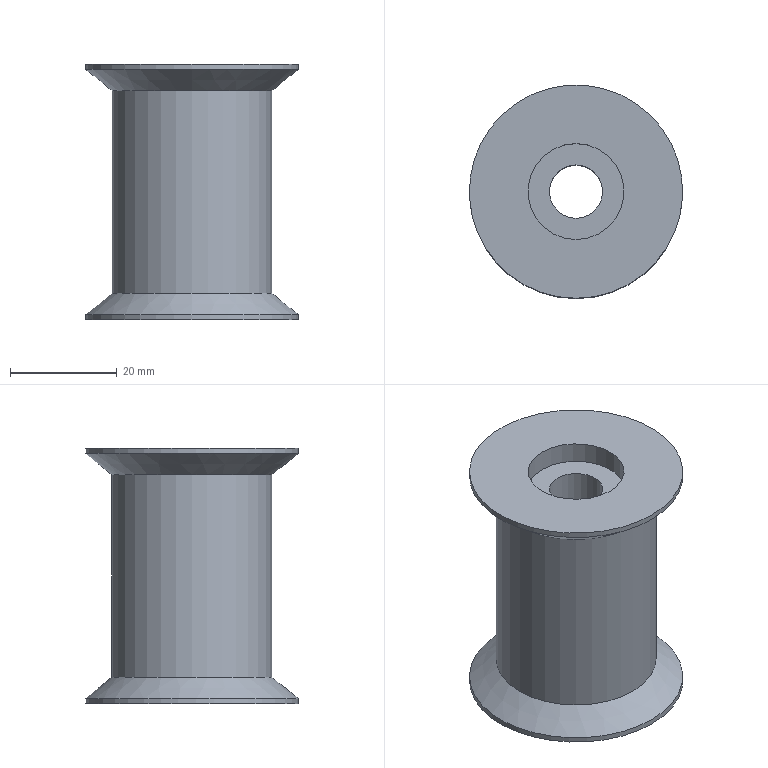Part | NX | features solid 2 | 1 solid | 10 faces | box 40 x 40 x 48 mm | volume 32650 mm3 | cylinder 5 | plane 3 | cone 2 | commonest cylinder face diameters 40 x2 10 x1 18 x1 30 x1
STEP:
#1=CARTESIAN_POINT('',(25.,-455.,-14.5));
#2=VERTEX_POINT('',#1);
#3=CARTESIAN_POINT('',(25.,-435.,-14.5));
#4=DIRECTION('',(0.,0.,-1.));
#5=DIRECTION('',(0.,-1.,0.));
#6=AXIS2_PLACEMENT_3D('',#3,#4,#5);
#7=CIRCLE('',#6,20.);
#8=EDGE_CURVE('',#2,#2,#7,.T.);
#9=ORIENTED_EDGE('',*,*,#8,.T.);
#10=EDGE_LOOP('',(#9));
#11=FACE_BOUND('',#10,.T.);
#12=CARTESIAN_POINT('',(25.,-440.,-14.5));
#13=VERTEX_POINT('',#12);
#14=CARTESIAN_POINT('',(25.,-435.,-14.5));
#15=DIRECTION('',(0.,0.,-1.));
#16=DIRECTION('',(0.,-1.,0.));
#17=AXIS2_PLACEMENT_3D('',#14,#15,#16);
#18=CIRCLE('',#17,5.);
#19=EDGE_CURVE('',#13,#13,#18,.F.);
#20=ORIENTED_EDGE('',*,*,#19,.T.);
#21=EDGE_LOOP('',(#20));
#22=FACE_BOUND('',#21,.T.);
#23=CARTESIAN_POINT('',(25.,-435.,-14.5));
#24=DIRECTION('',(0.,0.,-1.));
#25=DIRECTION('',(0.,-1.,0.));
#26=AXIS2_PLACEMENT_3D('',#23,#24,#25);
#27=PLANE('',#26);
#28=ADVANCED_FACE('',(#11,#22),#27,.T.);
#29=CARTESIAN_POINT('',(25.,-444.,29.5));
#30=VERTEX_POINT('',#29);
#31=CARTESIAN_POINT('',(25.,-435.,29.5));
#32=DIRECTION('',(0.,0.,-1.));
#33=DIRECTION('',(0.,-1.,0.));
#34=AXIS2_PLACEMENT_3D('',#31,#32,#33);
#35=CIRCLE('',#34,9.);
#36=EDGE_CURVE('',#30,#30,#35,.T.);
#37=ORIENTED_EDGE('',*,*,#36,.F.);
#38=EDGE_LOOP('',(#37));
#39=FACE_BOUND('',#38,.T.);
#40=CARTESIAN_POINT('',(25.,-440.,29.5));
#41=VERTEX_POINT('',#40);
#42=CARTESIAN_POINT('',(25.,-435.,29.5));
#43=DIRECTION('',(0.,0.,-1.));
#44=DIRECTION('',(0.,-1.,0.));
#45=AXIS2_PLACEMENT_3D('',#42,#43,#44);
#46=CIRCLE('',#45,5.);
#47=EDGE_CURVE('',#41,#41,#46,.T.);
#48=ORIENTED_EDGE('',*,*,#47,.T.);
#49=EDGE_LOOP('',(#48));
#50=FACE_BOUND('',#49,.T.);
#51=CARTESIAN_POINT('',(25.,-435.,29.5));
#52=DIRECTION('',(0.,0.,-1.));
#53=DIRECTION('',(0.,-1.,0.));
#54=AXIS2_PLACEMENT_3D('',#51,#52,#53);
#55=PLANE('',#54);
#56=ADVANCED_FACE('',(#39,#50),#55,.F.);
#57=CARTESIAN_POINT('',(25.,-455.,33.5));
#58=VERTEX_POINT('',#57);
#59=CARTESIAN_POINT('',(25.,-435.,33.5));
#60=DIRECTION('',(0.,0.,-1.));
#61=DIRECTION('',(0.,-1.,0.));
#62=AXIS2_PLACEMENT_3D('',#59,#60,#61);
#63=CIRCLE('',#62,20.);
#64=EDGE_CURVE('',#58,#58,#63,.T.);
#65=ORIENTED_EDGE('',*,*,#64,.F.);
#66=EDGE_LOOP('',(#65));
#67=FACE_BOUND('',#66,.T.);
#68=CARTESIAN_POINT('',(25.,-444.,33.5));
#69=VERTEX_POINT('',#68);
#70=CARTESIAN_POINT('',(25.,-435.,33.5));
#71=DIRECTION('',(0.,0.,-1.));
#72=DIRECTION('',(0.,-1.,0.));
#73=AXIS2_PLACEMENT_3D('',#70,#71,#72);
#74=CIRCLE('',#73,9.);
#75=EDGE_CURVE('',#69,#69,#74,.T.);
#76=ORIENTED_EDGE('',*,*,#75,.T.);
#77=EDGE_LOOP('',(#76));
#78=FACE_BOUND('',#77,.T.);
#79=CARTESIAN_POINT('',(25.,-435.,33.5));
#80=DIRECTION('',(0.,0.,-1.));
#81=DIRECTION('',(0.,-1.,0.));
#82=AXIS2_PLACEMENT_3D('',#79,#80,#81);
#83=PLANE('',#82);
#84=ADVANCED_FACE('',(#67,#78),#83,.F.);
#85=CARTESIAN_POINT('',(25.,-450.,28.5));
#86=VERTEX_POINT('',#85);
#87=CARTESIAN_POINT('',(25.,-435.,28.5));
#88=DIRECTION('',(0.,0.,-1.));
#89=DIRECTION('',(0.,-1.,0.));
#90=AXIS2_PLACEMENT_3D('',#87,#88,#89);
#91=CIRCLE('',#90,15.);
#92=EDGE_CURVE('',#86,#86,#91,.T.);
#93=ORIENTED_EDGE('',*,*,#92,.T.);
#94=EDGE_LOOP('',(#93));
#95=FACE_BOUND('',#94,.T.);
#96=CARTESIAN_POINT('',(25.,-450.,-9.5));
#97=VERTEX_POINT('',#96);
#98=CARTESIAN_POINT('',(25.,-435.,-9.5));
#99=DIRECTION('',(0.,0.,-1.));
#100=DIRECTION('',(0.,-1.,0.));
#101=AXIS2_PLACEMENT_3D('',#98,#99,#100);
#102=CIRCLE('',#101,15.);
#103=EDGE_CURVE('',#97,#97,#102,.F.);
#104=ORIENTED_EDGE('',*,*,#103,.T.);
#105=EDGE_LOOP('',(#104));
#106=FACE_BOUND('',#105,.T.);
#107=CARTESIAN_POINT('',(25.,-435.,-14.5));
#108=DIRECTION('',(0.,0.,1.));
#109=DIRECTION('',(0.,1.,0.));
#110=AXIS2_PLACEMENT_3D('',#107,#108,#109);
#111=CYLINDRICAL_SURFACE('',#110,15.);
#112=ADVANCED_FACE('',(#95,#106),#111,.T.);
#113=CARTESIAN_POINT('',(25.,-455.,-13.5));
#114=VERTEX_POINT('',#113);
#115=CARTESIAN_POINT('',(25.,-435.,-13.5));
#116=DIRECTION('',(0.,0.,-1.));
#117=DIRECTION('',(0.,-1.,0.));
#118=AXIS2_PLACEMENT_3D('',#115,#116,#117);
#119=CIRCLE('',#118,20.);
#120=EDGE_CURVE('',#114,#114,#119,.T.);
#121=ORIENTED_EDGE('',*,*,#120,.T.);
#122=EDGE_LOOP('',(#121));
#123=FACE_BOUND('',#122,.T.);
#124=ORIENTED_EDGE('',*,*,#8,.F.);
#125=EDGE_LOOP('',(#124));
#126=FACE_BOUND('',#125,.T.);
#127=CARTESIAN_POINT('',(25.,-435.,-14.5));
#128=DIRECTION('',(0.,0.,1.));
#129=DIRECTION('',(0.,1.,0.));
#130=AXIS2_PLACEMENT_3D('',#127,#128,#129);
#131=CYLINDRICAL_SURFACE('',#130,20.);
#132=ADVANCED_FACE('',(#123,#126),#131,.T.);
#133=ORIENTED_EDGE('',*,*,#103,.F.);
#134=EDGE_LOOP('',(#133));
#135=FACE_BOUND('',#134,.T.);
#136=ORIENTED_EDGE('',*,*,#120,.F.);
#137=EDGE_LOOP('',(#136));
#138=FACE_BOUND('',#137,.T.);
#139=CARTESIAN_POINT('',(25.,-435.,-13.5));
#140=DIRECTION('',(0.,0.,-1.));
#141=DIRECTION('',(0.,-1.,0.));
#142=AXIS2_PLACEMENT_3D('',#139,#140,#141);
#143=CONICAL_SURFACE('',#142,20.,0.8961);
#144=ADVANCED_FACE('',(#135,#138),#143,.T.);
#145=CARTESIAN_POINT('',(25.,-455.,32.5));
#146=VERTEX_POINT('',#145);
#147=CARTESIAN_POINT('',(25.,-435.,32.5));
#148=DIRECTION('',(0.,0.,-1.));
#149=DIRECTION('',(0.,-1.,0.));
#150=AXIS2_PLACEMENT_3D('',#147,#148,#149);
#151=CIRCLE('',#150,20.);
#152=EDGE_CURVE('',#146,#146,#151,.F.);
#153=ORIENTED_EDGE('',*,*,#152,.T.);
#154=EDGE_LOOP('',(#153));
#155=FACE_BOUND('',#154,.T.);
#156=ORIENTED_EDGE('',*,*,#64,.T.);
#157=EDGE_LOOP('',(#156));
#158=FACE_BOUND('',#157,.T.);
#159=CARTESIAN_POINT('',(25.,-435.,28.5));
#160=DIRECTION('',(0.,0.,1.));
#161=DIRECTION('',(0.,1.,0.));
#162=AXIS2_PLACEMENT_3D('',#159,#160,#161);
#163=CYLINDRICAL_SURFACE('',#162,20.);
#164=ADVANCED_FACE('',(#155,#158),#163,.T.);
#165=ORIENTED_EDGE('',*,*,#152,.F.);
#166=EDGE_LOOP('',(#165));
#167=FACE_BOUND('',#166,.T.);
#168=ORIENTED_EDGE('',*,*,#92,.F.);
#169=EDGE_LOOP('',(#168));
#170=FACE_BOUND('',#169,.T.);
#171=CARTESIAN_POINT('',(25.,-435.,28.5));
#172=DIRECTION('',(0.,0.,1.));
#173=DIRECTION('',(0.,1.,0.));
#174=AXIS2_PLACEMENT_3D('',#171,#172,#173);
#175=CONICAL_SURFACE('',#174,15.,0.8961);
#176=ADVANCED_FACE('',(#167,#170),#175,.T.);
#177=ORIENTED_EDGE('',*,*,#36,.T.);
#178=EDGE_LOOP('',(#177));
#179=FACE_BOUND('',#178,.T.);
#180=ORIENTED_EDGE('',*,*,#75,.F.);
#181=EDGE_LOOP('',(#180));
#182=FACE_BOUND('',#181,.T.);
#183=CARTESIAN_POINT('',(25.,-435.,29.5));
#184=DIRECTION('',(0.,0.,1.));
#185=DIRECTION('',(0.,1.,0.));
#186=AXIS2_PLACEMENT_3D('',#183,#184,#185);
#187=CYLINDRICAL_SURFACE('',#186,9.);
#188=ADVANCED_FACE('',(#179,#182),#187,.F.);
#189=ORIENTED_EDGE('',*,*,#19,.F.);
#190=EDGE_LOOP('',(#189));
#191=FACE_BOUND('',#190,.T.);
#192=ORIENTED_EDGE('',*,*,#47,.F.);
#193=EDGE_LOOP('',(#192));
#194=FACE_BOUND('',#193,.T.);
#195=CARTESIAN_POINT('',(25.,-435.,-35.));
#196=DIRECTION('',(0.,0.,1.));
#197=DIRECTION('',(0.,1.,0.));
#198=AXIS2_PLACEMENT_3D('',#195,#196,#197);
#199=CYLINDRICAL_SURFACE('',#198,5.);
#200=ADVANCED_FACE('',(#191,#194),#199,.F.);
#201=CLOSED_SHELL('',(#28,#56,#84,#112,#132,#144,#164,#176,#188,#200));
#202=MANIFOLD_SOLID_BREP('',#201);
#203=(LENGTH_UNIT()NAMED_UNIT(*)SI_UNIT(.MILLI.,.METRE.));
#204=UNCERTAINTY_MEASURE_WITH_UNIT(LENGTH_MEASURE(0.00001),#203,'','');
#205=(NAMED_UNIT(*)PLANE_ANGLE_UNIT()SI_UNIT($,.RADIAN.));
#206=(NAMED_UNIT(*)SI_UNIT($,.STERADIAN.)SOLID_ANGLE_UNIT());
#207=(GEOMETRIC_REPRESENTATION_CONTEXT(3)GLOBAL_UNCERTAINTY_ASSIGNED_CONTEXT((#204))GLOBAL_UNIT_ASSIGNED_CONTEXT((#203,#205,#206))REPRESENTATION_CONTEXT('',''));
#208=ADVANCED_BREP_SHAPE_REPRESENTATION('',(#202),#207);